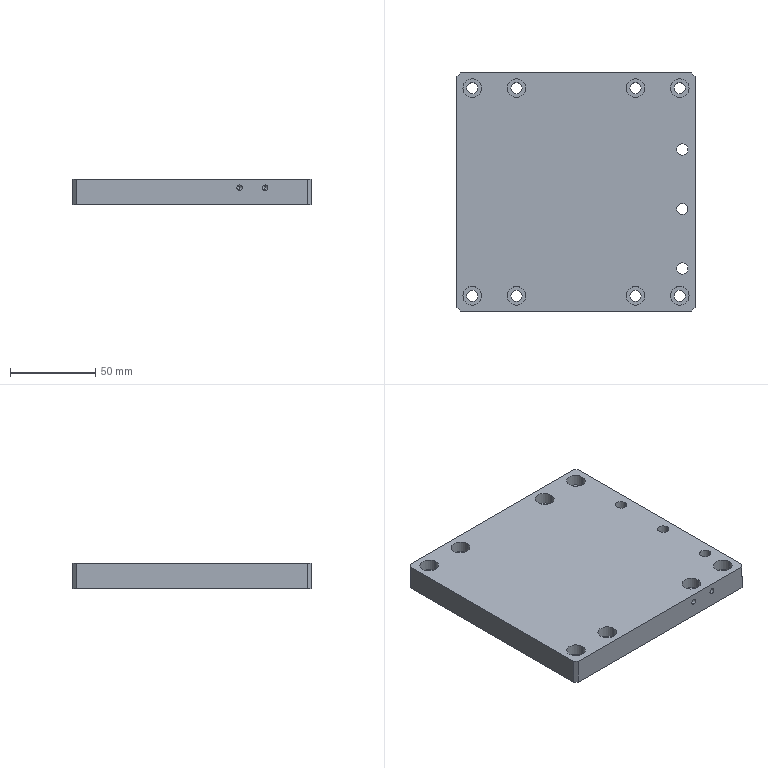Part | SolidWorks | features HoleWzd 3, Chamfer 1, Extrusion 1, LPattern 1, MirrorPattern 1 | 1 solid | 81 faces | box 140 x 140 x 15 mm | volume 283192 mm3 | cylinder 52 | plane 21 | cone 8 | commonest cylinder face diameters 6.6 x22 11 x22 3.3 x8